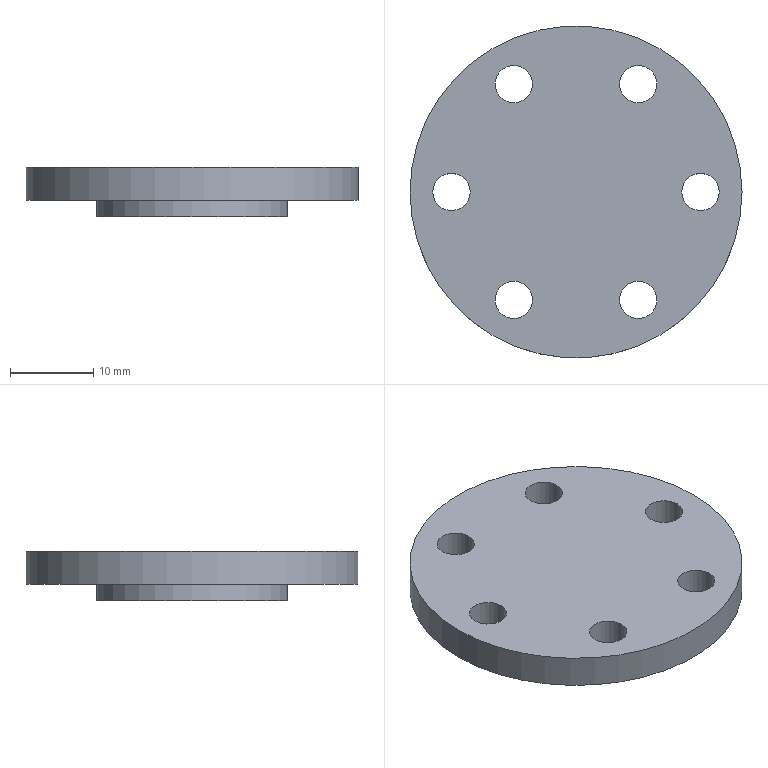Part | STEP file | zhouchenyagai2 | 1 solid | 13 faces | box 40 x 40 x 6 mm | volume 4909 mm3 | cylinder 9 | plane 4 | commonest cylinder face diameters 4.5 x6 19 x1 23 x1 40 x1
STEP:
#1=CARTESIAN_POINT('',(0.,0.,0.));
#2=DIRECTION('',(0.,0.,1.));
#3=DIRECTION('',(1.,0.,0.));
#4=AXIS2_PLACEMENT_3D('',#1,#2,#3);
#5=CARTESIAN_POINT('',(-9.75,12.99,4.));
#6=VERTEX_POINT('',#5);
#7=CARTESIAN_POINT('',(-7.5,12.99,4.));
#8=DIRECTION('',(0.,0.,-1.));
#9=DIRECTION('',(-1.,0.,0.));
#10=AXIS2_PLACEMENT_3D('',#7,#8,#9);
#11=CIRCLE('',#10,2.25);
#12=CARTESIAN_POINT('',(0.,0.,4.));
#13=DIRECTION('',(0.,0.,1.));
#14=DIRECTION('',(1.,0.,0.));
#15=AXIS2_PLACEMENT_3D('',#12,#13,#14);
#16=PLANE('',#15);
#17=CARTESIAN_POINT('',(-9.75,12.99));
#18=CARTESIAN_POINT('',(-9.75,16.887));
#19=CARTESIAN_POINT('',(-6.375,14.939));
#20=CARTESIAN_POINT('',(-3.,12.99));
#21=CARTESIAN_POINT('',(-6.375,11.042));
#22=CARTESIAN_POINT('',(-9.75,9.093));
#23=CARTESIAN_POINT('',(-9.75,12.99));
#24=(BOUNDED_CURVE()B_SPLINE_CURVE(2,(#17,#18,#19,#20,#21,#22,#23),.UNSPECIFIED.,.T.,.F.)B_SPLINE_CURVE_WITH_KNOTS((1,2,2,2,2,1),(-2.094,0.,2.094,4.189,6.283,8.378),.UNSPECIFIED.)CURVE()GEOMETRIC_REPRESENTATION_ITEM()RATIONAL_B_SPLINE_CURVE((1.,0.5,1.,0.5,1.,0.5,1.))REPRESENTATION_ITEM(''));
#25=(GEOMETRIC_REPRESENTATION_CONTEXT(2)PARAMETRIC_REPRESENTATION_CONTEXT()REPRESENTATION_CONTEXT('',''));
#26=DEFINITIONAL_REPRESENTATION('',(#24),#25);
#27=PCURVE('',#16,#26);
#28=CARTESIAN_POINT('',(-7.5,12.99,4.));
#29=DIRECTION('',(0.,0.,-1.));
#30=DIRECTION('',(-1.,0.,0.));
#31=AXIS2_PLACEMENT_3D('',#28,#29,#30);
#32=CYLINDRICAL_SURFACE('',#31,2.25);
#33=CARTESIAN_POINT('',(0.,0.));
#34=DIRECTION('',(1.,0.));
#35=VECTOR('',#34,1.);
#36=LINE('',#33,#35);
#37=(GEOMETRIC_REPRESENTATION_CONTEXT(2)PARAMETRIC_REPRESENTATION_CONTEXT()REPRESENTATION_CONTEXT('',''));
#38=DEFINITIONAL_REPRESENTATION('',(#36),#37);
#39=PCURVE('',#32,#38);
#40=SURFACE_CURVE('',#11,(#27,#39),.PCURVE_S1.);
#41=EDGE_CURVE('',#6,#6,#40,.T.);
#42=ORIENTED_EDGE('',*,*,#41,.T.);
#43=EDGE_LOOP('',(#42));
#44=FACE_BOUND('',#43,.T.);
#45=CARTESIAN_POINT('',(12.75,0.,4.));
#46=VERTEX_POINT('',#45);
#47=CARTESIAN_POINT('',(15.,0.,4.));
#48=DIRECTION('',(0.,0.,-1.));
#49=DIRECTION('',(-1.,0.,0.));
#50=AXIS2_PLACEMENT_3D('',#47,#48,#49);
#51=CIRCLE('',#50,2.25);
#52=CARTESIAN_POINT('',(12.75,0.));
#53=CARTESIAN_POINT('',(12.75,3.897));
#54=CARTESIAN_POINT('',(16.125,1.949));
#55=CARTESIAN_POINT('',(19.5,0.));
#56=CARTESIAN_POINT('',(16.125,-1.949));
#57=CARTESIAN_POINT('',(12.75,-3.897));
#58=CARTESIAN_POINT('',(12.75,0.));
#59=(BOUNDED_CURVE()B_SPLINE_CURVE(2,(#52,#53,#54,#55,#56,#57,#58),.UNSPECIFIED.,.T.,.F.)B_SPLINE_CURVE_WITH_KNOTS((1,2,2,2,2,1),(-2.094,0.,2.094,4.189,6.283,8.378),.UNSPECIFIED.)CURVE()GEOMETRIC_REPRESENTATION_ITEM()RATIONAL_B_SPLINE_CURVE((1.,0.5,1.,0.5,1.,0.5,1.))REPRESENTATION_ITEM(''));
#60=(GEOMETRIC_REPRESENTATION_CONTEXT(2)PARAMETRIC_REPRESENTATION_CONTEXT()REPRESENTATION_CONTEXT('',''));
#61=DEFINITIONAL_REPRESENTATION('',(#59),#60);
#62=PCURVE('',#16,#61);
#63=CARTESIAN_POINT('',(15.,0.,4.));
#64=DIRECTION('',(0.,0.,-1.));
#65=DIRECTION('',(-1.,0.,0.));
#66=AXIS2_PLACEMENT_3D('',#63,#64,#65);
#67=CYLINDRICAL_SURFACE('',#66,2.25);
#68=CARTESIAN_POINT('',(0.,0.));
#69=DIRECTION('',(1.,0.));
#70=VECTOR('',#69,1.);
#71=LINE('',#68,#70);
#72=(GEOMETRIC_REPRESENTATION_CONTEXT(2)PARAMETRIC_REPRESENTATION_CONTEXT()REPRESENTATION_CONTEXT('',''));
#73=DEFINITIONAL_REPRESENTATION('',(#71),#72);
#74=PCURVE('',#67,#73);
#75=SURFACE_CURVE('',#51,(#62,#74),.PCURVE_S1.);
#76=EDGE_CURVE('',#46,#46,#75,.T.);
#77=ORIENTED_EDGE('',*,*,#76,.T.);
#78=EDGE_LOOP('',(#77));
#79=FACE_BOUND('',#78,.T.);
#80=CARTESIAN_POINT('',(-9.75,-12.99,4.));
#81=VERTEX_POINT('',#80);
#82=CARTESIAN_POINT('',(-7.5,-12.99,4.));
#83=DIRECTION('',(0.,0.,-1.));
#84=DIRECTION('',(-1.,0.,0.));
#85=AXIS2_PLACEMENT_3D('',#82,#83,#84);
#86=CIRCLE('',#85,2.25);
#87=CARTESIAN_POINT('',(-9.75,-12.99));
#88=CARTESIAN_POINT('',(-9.75,-9.093));
#89=CARTESIAN_POINT('',(-6.375,-11.042));
#90=CARTESIAN_POINT('',(-3.,-12.99));
#91=CARTESIAN_POINT('',(-6.375,-14.939));
#92=CARTESIAN_POINT('',(-9.75,-16.887));
#93=CARTESIAN_POINT('',(-9.75,-12.99));
#94=(BOUNDED_CURVE()B_SPLINE_CURVE(2,(#87,#88,#89,#90,#91,#92,#93),.UNSPECIFIED.,.T.,.F.)B_SPLINE_CURVE_WITH_KNOTS((1,2,2,2,2,1),(-2.094,0.,2.094,4.189,6.283,8.378),.UNSPECIFIED.)CURVE()GEOMETRIC_REPRESENTATION_ITEM()RATIONAL_B_SPLINE_CURVE((1.,0.5,1.,0.5,1.,0.5,1.))REPRESENTATION_ITEM(''));
#95=(GEOMETRIC_REPRESENTATION_CONTEXT(2)PARAMETRIC_REPRESENTATION_CONTEXT()REPRESENTATION_CONTEXT('',''));
#96=DEFINITIONAL_REPRESENTATION('',(#94),#95);
#97=PCURVE('',#16,#96);
#98=CARTESIAN_POINT('',(-7.5,-12.99,4.));
#99=DIRECTION('',(0.,0.,-1.));
#100=DIRECTION('',(-1.,0.,0.));
#101=AXIS2_PLACEMENT_3D('',#98,#99,#100);
#102=CYLINDRICAL_SURFACE('',#101,2.25);
#103=CARTESIAN_POINT('',(0.,0.));
#104=DIRECTION('',(1.,0.));
#105=VECTOR('',#104,1.);
#106=LINE('',#103,#105);
#107=(GEOMETRIC_REPRESENTATION_CONTEXT(2)PARAMETRIC_REPRESENTATION_CONTEXT()REPRESENTATION_CONTEXT('',''));
#108=DEFINITIONAL_REPRESENTATION('',(#106),#107);
#109=PCURVE('',#102,#108);
#110=SURFACE_CURVE('',#86,(#97,#109),.PCURVE_S1.);
#111=EDGE_CURVE('',#81,#81,#110,.T.);
#112=ORIENTED_EDGE('',*,*,#111,.T.);
#113=EDGE_LOOP('',(#112));
#114=FACE_BOUND('',#113,.T.);
#115=CARTESIAN_POINT('',(-20.,0.,4.));
#116=VERTEX_POINT('',#115);
#117=CARTESIAN_POINT('',(0.,0.,4.));
#118=DIRECTION('',(0.,0.,1.));
#119=DIRECTION('',(-1.,0.,0.));
#120=AXIS2_PLACEMENT_3D('',#117,#118,#119);
#121=CIRCLE('',#120,20.);
#122=CARTESIAN_POINT('',(0.,0.));
#123=DIRECTION('',(-1.,0.));
#124=AXIS2_PLACEMENT_2D('',#122,#123);
#125=CIRCLE('',#124,20.);
#126=(GEOMETRIC_REPRESENTATION_CONTEXT(2)PARAMETRIC_REPRESENTATION_CONTEXT()REPRESENTATION_CONTEXT('',''));
#127=DEFINITIONAL_REPRESENTATION('',(#125),#126);
#128=PCURVE('',#16,#127);
#129=CARTESIAN_POINT('',(0.,0.,4.));
#130=DIRECTION('',(0.,0.,-1.));
#131=DIRECTION('',(-1.,0.,0.));
#132=AXIS2_PLACEMENT_3D('',#129,#130,#131);
#133=CYLINDRICAL_SURFACE('',#132,20.);
#134=CARTESIAN_POINT('',(6.283,0.));
#135=DIRECTION('',(-1.,0.));
#136=VECTOR('',#135,1.);
#137=LINE('',#134,#136);
#138=(GEOMETRIC_REPRESENTATION_CONTEXT(2)PARAMETRIC_REPRESENTATION_CONTEXT()REPRESENTATION_CONTEXT('',''));
#139=DEFINITIONAL_REPRESENTATION('',(#137),#138);
#140=PCURVE('',#133,#139);
#141=SURFACE_CURVE('',#121,(#128,#140),.PCURVE_S1.);
#142=EDGE_CURVE('',#116,#116,#141,.T.);
#143=ORIENTED_EDGE('',*,*,#142,.T.);
#144=EDGE_LOOP('',(#143));
#145=FACE_BOUND('',#144,.T.);
#146=CARTESIAN_POINT('',(-17.25,0.,4.));
#147=VERTEX_POINT('',#146);
#148=CARTESIAN_POINT('',(-15.,0.,4.));
#149=DIRECTION('',(0.,0.,-1.));
#150=DIRECTION('',(-1.,0.,0.));
#151=AXIS2_PLACEMENT_3D('',#148,#149,#150);
#152=CIRCLE('',#151,2.25);
#153=CARTESIAN_POINT('',(-17.25,0.));
#154=CARTESIAN_POINT('',(-17.25,3.897));
#155=CARTESIAN_POINT('',(-13.875,1.949));
#156=CARTESIAN_POINT('',(-10.5,0.));
#157=CARTESIAN_POINT('',(-13.875,-1.949));
#158=CARTESIAN_POINT('',(-17.25,-3.897));
#159=CARTESIAN_POINT('',(-17.25,0.));
#160=(BOUNDED_CURVE()B_SPLINE_CURVE(2,(#153,#154,#155,#156,#157,#158,#159),.UNSPECIFIED.,.T.,.F.)B_SPLINE_CURVE_WITH_KNOTS((1,2,2,2,2,1),(-2.094,0.,2.094,4.189,6.283,8.378),.UNSPECIFIED.)CURVE()GEOMETRIC_REPRESENTATION_ITEM()RATIONAL_B_SPLINE_CURVE((1.,0.5,1.,0.5,1.,0.5,1.))REPRESENTATION_ITEM(''));
#161=(GEOMETRIC_REPRESENTATION_CONTEXT(2)PARAMETRIC_REPRESENTATION_CONTEXT()REPRESENTATION_CONTEXT('',''));
#162=DEFINITIONAL_REPRESENTATION('',(#160),#161);
#163=PCURVE('',#16,#162);
#164=CARTESIAN_POINT('',(-15.,0.,4.));
#165=DIRECTION('',(0.,0.,-1.));
#166=DIRECTION('',(-1.,0.,0.));
#167=AXIS2_PLACEMENT_3D('',#164,#165,#166);
#168=CYLINDRICAL_SURFACE('',#167,2.25);
#169=CARTESIAN_POINT('',(0.,0.));
#170=DIRECTION('',(1.,0.));
#171=VECTOR('',#170,1.);
#172=LINE('',#169,#171);
#173=(GEOMETRIC_REPRESENTATION_CONTEXT(2)PARAMETRIC_REPRESENTATION_CONTEXT()REPRESENTATION_CONTEXT('',''));
#174=DEFINITIONAL_REPRESENTATION('',(#172),#173);
#175=PCURVE('',#168,#174);
#176=SURFACE_CURVE('',#152,(#163,#175),.PCURVE_S1.);
#177=EDGE_CURVE('',#147,#147,#176,.T.);
#178=ORIENTED_EDGE('',*,*,#177,.T.);
#179=EDGE_LOOP('',(#178));
#180=FACE_BOUND('',#179,.T.);
#181=CARTESIAN_POINT('',(5.25,-12.99,4.));
#182=VERTEX_POINT('',#181);
#183=CARTESIAN_POINT('',(7.5,-12.99,4.));
#184=DIRECTION('',(0.,0.,-1.));
#185=DIRECTION('',(-1.,0.,0.));
#186=AXIS2_PLACEMENT_3D('',#183,#184,#185);
#187=CIRCLE('',#186,2.25);
#188=CARTESIAN_POINT('',(5.25,-12.99));
#189=CARTESIAN_POINT('',(5.25,-9.093));
#190=CARTESIAN_POINT('',(8.625,-11.042));
#191=CARTESIAN_POINT('',(12.,-12.99));
#192=CARTESIAN_POINT('',(8.625,-14.939));
#193=CARTESIAN_POINT('',(5.25,-16.887));
#194=CARTESIAN_POINT('',(5.25,-12.99));
#195=(BOUNDED_CURVE()B_SPLINE_CURVE(2,(#188,#189,#190,#191,#192,#193,#194),.UNSPECIFIED.,.T.,.F.)B_SPLINE_CURVE_WITH_KNOTS((1,2,2,2,2,1),(-2.094,0.,2.094,4.189,6.283,8.378),.UNSPECIFIED.)CURVE()GEOMETRIC_REPRESENTATION_ITEM()RATIONAL_B_SPLINE_CURVE((1.,0.5,1.,0.5,1.,0.5,1.))REPRESENTATION_ITEM(''));
#196=(GEOMETRIC_REPRESENTATION_CONTEXT(2)PARAMETRIC_REPRESENTATION_CONTEXT()REPRESENTATION_CONTEXT('',''));
#197=DEFINITIONAL_REPRESENTATION('',(#195),#196);
#198=PCURVE('',#16,#197);
#199=CARTESIAN_POINT('',(7.5,-12.99,4.));
#200=DIRECTION('',(0.,0.,-1.));
#201=DIRECTION('',(-1.,0.,0.));
#202=AXIS2_PLACEMENT_3D('',#199,#200,#201);
#203=CYLINDRICAL_SURFACE('',#202,2.25);
#204=CARTESIAN_POINT('',(0.,0.));
#205=DIRECTION('',(1.,0.));
#206=VECTOR('',#205,1.);
#207=LINE('',#204,#206);
#208=(GEOMETRIC_REPRESENTATION_CONTEXT(2)PARAMETRIC_REPRESENTATION_CONTEXT()REPRESENTATION_CONTEXT('',''));
#209=DEFINITIONAL_REPRESENTATION('',(#207),#208);
#210=PCURVE('',#203,#209);
#211=SURFACE_CURVE('',#187,(#198,#210),.PCURVE_S1.);
#212=EDGE_CURVE('',#182,#182,#211,.T.);
#213=ORIENTED_EDGE('',*,*,#212,.T.);
#214=EDGE_LOOP('',(#213));
#215=FACE_BOUND('',#214,.T.);
#216=CARTESIAN_POINT('',(5.25,12.99,4.));
#217=VERTEX_POINT('',#216);
#218=CARTESIAN_POINT('',(7.5,12.99,4.));
#219=DIRECTION('',(0.,0.,-1.));
#220=DIRECTION('',(-1.,0.,0.));
#221=AXIS2_PLACEMENT_3D('',#218,#219,#220);
#222=CIRCLE('',#221,2.25);
#223=CARTESIAN_POINT('',(5.25,12.99));
#224=CARTESIAN_POINT('',(5.25,16.887));
#225=CARTESIAN_POINT('',(8.625,14.939));
#226=CARTESIAN_POINT('',(12.,12.99));
#227=CARTESIAN_POINT('',(8.625,11.042));
#228=CARTESIAN_POINT('',(5.25,9.093));
#229=CARTESIAN_POINT('',(5.25,12.99));
#230=(BOUNDED_CURVE()B_SPLINE_CURVE(2,(#223,#224,#225,#226,#227,#228,#229),.UNSPECIFIED.,.T.,.F.)B_SPLINE_CURVE_WITH_KNOTS((1,2,2,2,2,1),(-2.094,0.,2.094,4.189,6.283,8.378),.UNSPECIFIED.)CURVE()GEOMETRIC_REPRESENTATION_ITEM()RATIONAL_B_SPLINE_CURVE((1.,0.5,1.,0.5,1.,0.5,1.))REPRESENTATION_ITEM(''));
#231=(GEOMETRIC_REPRESENTATION_CONTEXT(2)PARAMETRIC_REPRESENTATION_CONTEXT()REPRESENTATION_CONTEXT('',''));
#232=DEFINITIONAL_REPRESENTATION('',(#230),#231);
#233=PCURVE('',#16,#232);
#234=CARTESIAN_POINT('',(7.5,12.99,4.));
#235=DIRECTION('',(0.,0.,-1.));
#236=DIRECTION('',(-1.,0.,0.));
#237=AXIS2_PLACEMENT_3D('',#234,#235,#236);
#238=CYLINDRICAL_SURFACE('',#237,2.25);
#239=CARTESIAN_POINT('',(0.,0.));
#240=DIRECTION('',(1.,0.));
#241=VECTOR('',#240,1.);
#242=LINE('',#239,#241);
#243=(GEOMETRIC_REPRESENTATION_CONTEXT(2)PARAMETRIC_REPRESENTATION_CONTEXT()REPRESENTATION_CONTEXT('',''));
#244=DEFINITIONAL_REPRESENTATION('',(#242),#243);
#245=PCURVE('',#238,#244);
#246=SURFACE_CURVE('',#222,(#233,#245),.PCURVE_S1.);
#247=EDGE_CURVE('',#217,#217,#246,.T.);
#248=ORIENTED_EDGE('',*,*,#247,.T.);
#249=EDGE_LOOP('',(#248));
#250=FACE_BOUND('',#249,.T.);
#251=ADVANCED_FACE('',(#44,#79,#114,#145,#180,#215,#250),#16,.T.);
#252=ORIENTED_EDGE('',*,*,#41,.T.);
#253=CARTESIAN_POINT('',(-9.75,12.99,0.));
#254=VERTEX_POINT('',#253);
#255=CARTESIAN_POINT('',(-9.75,12.99,4.));
#256=CARTESIAN_POINT('',(-9.75,12.99,0.));
#257=B_SPLINE_CURVE_WITH_KNOTS('',1,(#255,#256),.UNSPECIFIED.,.F.,.F.,(2,2),(0.,4.),.PIECEWISE_BEZIER_KNOTS.);
#258=CARTESIAN_POINT('',(6.283,0.));
#259=DIRECTION('',(0.,1.));
#260=VECTOR('',#259,1.);
#261=LINE('',#258,#260);
#262=(GEOMETRIC_REPRESENTATION_CONTEXT(2)PARAMETRIC_REPRESENTATION_CONTEXT()REPRESENTATION_CONTEXT('',''));
#263=DEFINITIONAL_REPRESENTATION('',(#261),#262);
#264=PCURVE('',#32,#263);
#265=CARTESIAN_POINT('',(0.,0.));
#266=DIRECTION('',(0.,1.));
#267=VECTOR('',#266,1.);
#268=LINE('',#265,#267);
#269=(GEOMETRIC_REPRESENTATION_CONTEXT(2)PARAMETRIC_REPRESENTATION_CONTEXT()REPRESENTATION_CONTEXT('',''));
#270=DEFINITIONAL_REPRESENTATION('',(#268),#269);
#271=PCURVE('',#32,#270);
#272=SEAM_CURVE('',#257,(#264,#271),.PCURVE_S1.);
#273=EDGE_CURVE('',#6,#254,#272,.T.);
#274=ORIENTED_EDGE('',*,*,#273,.T.);
#275=CARTESIAN_POINT('',(-7.5,12.99,0.));
#276=DIRECTION('',(0.,0.,1.));
#277=DIRECTION('',(-1.,0.,0.));
#278=AXIS2_PLACEMENT_3D('',#275,#276,#277);
#279=CIRCLE('',#278,2.25);
#280=CARTESIAN_POINT('',(6.283,4.));
#281=DIRECTION('',(-1.,0.));
#282=VECTOR('',#281,1.);
#283=LINE('',#280,#282);
#284=(GEOMETRIC_REPRESENTATION_CONTEXT(2)PARAMETRIC_REPRESENTATION_CONTEXT()REPRESENTATION_CONTEXT('',''));
#285=DEFINITIONAL_REPRESENTATION('',(#283),#284);
#286=PCURVE('',#32,#285);
#287=CARTESIAN_POINT('',(0.,0.,0.));
#288=DIRECTION('',(0.,0.,1.));
#289=DIRECTION('',(1.,0.,0.));
#290=AXIS2_PLACEMENT_3D('',#287,#288,#289);
#291=PLANE('',#290);
#292=CARTESIAN_POINT('',(-7.5,12.99));
#293=DIRECTION('',(-1.,0.));
#294=AXIS2_PLACEMENT_2D('',#292,#293);
#295=CIRCLE('',#294,2.25);
#296=(GEOMETRIC_REPRESENTATION_CONTEXT(2)PARAMETRIC_REPRESENTATION_CONTEXT()REPRESENTATION_CONTEXT('',''));
#297=DEFINITIONAL_REPRESENTATION('',(#295),#296);
#298=PCURVE('',#291,#297);
#299=SURFACE_CURVE('',#279,(#286,#298),.PCURVE_S1.);
#300=EDGE_CURVE('',#254,#254,#299,.T.);
#301=ORIENTED_EDGE('',*,*,#300,.T.);
#302=ORIENTED_EDGE('',*,*,#273,.F.);
#303=EDGE_LOOP('',(#252,#274,#301,#302));
#304=FACE_BOUND('',#303,.F.);
#305=ADVANCED_FACE('',(#304),#32,.F.);
#306=ORIENTED_EDGE('',*,*,#76,.T.);
#307=CARTESIAN_POINT('',(12.75,0.,0.));
#308=VERTEX_POINT('',#307);
#309=CARTESIAN_POINT('',(12.75,0.,4.));
#310=CARTESIAN_POINT('',(12.75,0.,0.));
#311=B_SPLINE_CURVE_WITH_KNOTS('',1,(#309,#310),.UNSPECIFIED.,.F.,.F.,(2,2),(0.,4.),.PIECEWISE_BEZIER_KNOTS.);
#312=CARTESIAN_POINT('',(6.283,0.));
#313=DIRECTION('',(0.,1.));
#314=VECTOR('',#313,1.);
#315=LINE('',#312,#314);
#316=(GEOMETRIC_REPRESENTATION_CONTEXT(2)PARAMETRIC_REPRESENTATION_CONTEXT()REPRESENTATION_CONTEXT('',''));
#317=DEFINITIONAL_REPRESENTATION('',(#315),#316);
#318=PCURVE('',#67,#317);
#319=CARTESIAN_POINT('',(0.,0.));
#320=DIRECTION('',(0.,1.));
#321=VECTOR('',#320,1.);
#322=LINE('',#319,#321);
#323=(GEOMETRIC_REPRESENTATION_CONTEXT(2)PARAMETRIC_REPRESENTATION_CONTEXT()REPRESENTATION_CONTEXT('',''));
#324=DEFINITIONAL_REPRESENTATION('',(#322),#323);
#325=PCURVE('',#67,#324);
#326=SEAM_CURVE('',#311,(#318,#325),.PCURVE_S1.);
#327=EDGE_CURVE('',#46,#308,#326,.T.);
#328=ORIENTED_EDGE('',*,*,#327,.T.);
#329=CARTESIAN_POINT('',(15.,0.,0.));
#330=DIRECTION('',(0.,0.,1.));
#331=DIRECTION('',(-1.,0.,0.));
#332=AXIS2_PLACEMENT_3D('',#329,#330,#331);
#333=CIRCLE('',#332,2.25);
#334=CARTESIAN_POINT('',(6.283,4.));
#335=DIRECTION('',(-1.,0.));
#336=VECTOR('',#335,1.);
#337=LINE('',#334,#336);
#338=(GEOMETRIC_REPRESENTATION_CONTEXT(2)PARAMETRIC_REPRESENTATION_CONTEXT()REPRESENTATION_CONTEXT('',''));
#339=DEFINITIONAL_REPRESENTATION('',(#337),#338);
#340=PCURVE('',#67,#339);
#341=CARTESIAN_POINT('',(15.,0.));
#342=DIRECTION('',(-1.,0.));
#343=AXIS2_PLACEMENT_2D('',#341,#342);
#344=CIRCLE('',#343,2.25);
#345=(GEOMETRIC_REPRESENTATION_CONTEXT(2)PARAMETRIC_REPRESENTATION_CONTEXT()REPRESENTATION_CONTEXT('',''));
#346=DEFINITIONAL_REPRESENTATION('',(#344),#345);
#347=PCURVE('',#291,#346);
#348=SURFACE_CURVE('',#333,(#340,#347),.PCURVE_S1.);
#349=EDGE_CURVE('',#308,#308,#348,.T.);
#350=ORIENTED_EDGE('',*,*,#349,.T.);
#351=ORIENTED_EDGE('',*,*,#327,.F.);
#352=EDGE_LOOP('',(#306,#328,#350,#351));
#353=FACE_BOUND('',#352,.F.);
#354=ADVANCED_FACE('',(#353),#67,.F.);
#355=ORIENTED_EDGE('',*,*,#111,.T.);
#356=CARTESIAN_POINT('',(-9.75,-12.99,0.));
#357=VERTEX_POINT('',#356);
#358=CARTESIAN_POINT('',(-9.75,-12.99,4.));
#359=CARTESIAN_POINT('',(-9.75,-12.99,0.));
#360=B_SPLINE_CURVE_WITH_KNOTS('',1,(#358,#359),.UNSPECIFIED.,.F.,.F.,(2,2),(0.,4.),.PIECEWISE_BEZIER_KNOTS.);
#361=CARTESIAN_POINT('',(6.283,0.));
#362=DIRECTION('',(0.,1.));
#363=VECTOR('',#362,1.);
#364=LINE('',#361,#363);
#365=(GEOMETRIC_REPRESENTATION_CONTEXT(2)PARAMETRIC_REPRESENTATION_CONTEXT()REPRESENTATION_CONTEXT('',''));
#366=DEFINITIONAL_REPRESENTATION('',(#364),#365);
#367=PCURVE('',#102,#366);
#368=CARTESIAN_POINT('',(0.,0.));
#369=DIRECTION('',(0.,1.));
#370=VECTOR('',#369,1.);
#371=LINE('',#368,#370);
#372=(GEOMETRIC_REPRESENTATION_CONTEXT(2)PARAMETRIC_REPRESENTATION_CONTEXT()REPRESENTATION_CONTEXT('',''));
#373=DEFINITIONAL_REPRESENTATION('',(#371),#372);
#374=PCURVE('',#102,#373);
#375=SEAM_CURVE('',#360,(#367,#374),.PCURVE_S1.);
#376=EDGE_CURVE('',#81,#357,#375,.T.);
#377=ORIENTED_EDGE('',*,*,#376,.T.);
#378=CARTESIAN_POINT('',(-7.5,-12.99,0.));
#379=DIRECTION('',(0.,0.,1.));
#380=DIRECTION('',(-1.,0.,0.));
#381=AXIS2_PLACEMENT_3D('',#378,#379,#380);
#382=CIRCLE('',#381,2.25);
#383=CARTESIAN_POINT('',(6.283,4.));
#384=DIRECTION('',(-1.,0.));
#385=VECTOR('',#384,1.);
#386=LINE('',#383,#385);
#387=(GEOMETRIC_REPRESENTATION_CONTEXT(2)PARAMETRIC_REPRESENTATION_CONTEXT()REPRESENTATION_CONTEXT('',''));
#388=DEFINITIONAL_REPRESENTATION('',(#386),#387);
#389=PCURVE('',#102,#388);
#390=CARTESIAN_POINT('',(-7.5,-12.99));
#391=DIRECTION('',(-1.,0.));
#392=AXIS2_PLACEMENT_2D('',#390,#391);
#393=CIRCLE('',#392,2.25);
#394=(GEOMETRIC_REPRESENTATION_CONTEXT(2)PARAMETRIC_REPRESENTATION_CONTEXT()REPRESENTATION_CONTEXT('',''));
#395=DEFINITIONAL_REPRESENTATION('',(#393),#394);
#396=PCURVE('',#291,#395);
#397=SURFACE_CURVE('',#382,(#389,#396),.PCURVE_S1.);
#398=EDGE_CURVE('',#357,#357,#397,.T.);
#399=ORIENTED_EDGE('',*,*,#398,.T.);
#400=ORIENTED_EDGE('',*,*,#376,.F.);
#401=EDGE_LOOP('',(#355,#377,#399,#400));
#402=FACE_BOUND('',#401,.F.);
#403=ADVANCED_FACE('',(#402),#102,.F.);
#404=CARTESIAN_POINT('',(-20.,0.,0.));
#405=VERTEX_POINT('',#404);
#406=CARTESIAN_POINT('',(0.,0.,0.));
#407=DIRECTION('',(0.,0.,1.));
#408=DIRECTION('',(-1.,0.,0.));
#409=AXIS2_PLACEMENT_3D('',#406,#407,#408);
#410=CIRCLE('',#409,20.);
#411=CARTESIAN_POINT('',(6.283,4.));
#412=DIRECTION('',(-1.,0.));
#413=VECTOR('',#412,1.);
#414=LINE('',#411,#413);
#415=(GEOMETRIC_REPRESENTATION_CONTEXT(2)PARAMETRIC_REPRESENTATION_CONTEXT()REPRESENTATION_CONTEXT('',''));
#416=DEFINITIONAL_REPRESENTATION('',(#414),#415);
#417=PCURVE('',#133,#416);
#418=CARTESIAN_POINT('',(0.,0.));
#419=DIRECTION('',(-1.,0.));
#420=AXIS2_PLACEMENT_2D('',#418,#419);
#421=CIRCLE('',#420,20.);
#422=(GEOMETRIC_REPRESENTATION_CONTEXT(2)PARAMETRIC_REPRESENTATION_CONTEXT()REPRESENTATION_CONTEXT('',''));
#423=DEFINITIONAL_REPRESENTATION('',(#421),#422);
#424=PCURVE('',#291,#423);
#425=SURFACE_CURVE('',#410,(#417,#424),.PCURVE_S1.);
#426=EDGE_CURVE('',#405,#405,#425,.T.);
#427=ORIENTED_EDGE('',*,*,#426,.T.);
#428=CARTESIAN_POINT('',(-20.,0.,4.));
#429=CARTESIAN_POINT('',(-20.,0.,0.));
#430=B_SPLINE_CURVE_WITH_KNOTS('',1,(#428,#429),.UNSPECIFIED.,.F.,.F.,(2,2),(0.,4.),.PIECEWISE_BEZIER_KNOTS.);
#431=CARTESIAN_POINT('',(0.,0.));
#432=DIRECTION('',(0.,1.));
#433=VECTOR('',#432,1.);
#434=LINE('',#431,#433);
#435=(GEOMETRIC_REPRESENTATION_CONTEXT(2)PARAMETRIC_REPRESENTATION_CONTEXT()REPRESENTATION_CONTEXT('',''));
#436=DEFINITIONAL_REPRESENTATION('',(#434),#435);
#437=PCURVE('',#133,#436);
#438=CARTESIAN_POINT('',(6.283,0.));
#439=DIRECTION('',(0.,1.));
#440=VECTOR('',#439,1.);
#441=LINE('',#438,#440);
#442=(GEOMETRIC_REPRESENTATION_CONTEXT(2)PARAMETRIC_REPRESENTATION_CONTEXT()REPRESENTATION_CONTEXT('',''));
#443=DEFINITIONAL_REPRESENTATION('',(#441),#442);
#444=PCURVE('',#133,#443);
#445=SEAM_CURVE('',#430,(#437,#444),.PCURVE_S1.);
#446=EDGE_CURVE('',#116,#405,#445,.T.);
#447=ORIENTED_EDGE('',*,*,#446,.F.);
#448=ORIENTED_EDGE('',*,*,#142,.F.);
#449=ORIENTED_EDGE('',*,*,#446,.T.);
#450=EDGE_LOOP('',(#427,#447,#448,#449));
#451=FACE_BOUND('',#450,.T.);
#452=ADVANCED_FACE('',(#451),#133,.T.);
#453=ORIENTED_EDGE('',*,*,#177,.T.);
#454=CARTESIAN_POINT('',(-17.25,0.,0.));
#455=VERTEX_POINT('',#454);
#456=CARTESIAN_POINT('',(-17.25,0.,4.));
#457=CARTESIAN_POINT('',(-17.25,0.,0.));
#458=B_SPLINE_CURVE_WITH_KNOTS('',1,(#456,#457),.UNSPECIFIED.,.F.,.F.,(2,2),(0.,4.),.PIECEWISE_BEZIER_KNOTS.);
#459=CARTESIAN_POINT('',(6.283,0.));
#460=DIRECTION('',(0.,1.));
#461=VECTOR('',#460,1.);
#462=LINE('',#459,#461);
#463=(GEOMETRIC_REPRESENTATION_CONTEXT(2)PARAMETRIC_REPRESENTATION_CONTEXT()REPRESENTATION_CONTEXT('',''));
#464=DEFINITIONAL_REPRESENTATION('',(#462),#463);
#465=PCURVE('',#168,#464);
#466=CARTESIAN_POINT('',(0.,0.));
#467=DIRECTION('',(0.,1.));
#468=VECTOR('',#467,1.);
#469=LINE('',#466,#468);
#470=(GEOMETRIC_REPRESENTATION_CONTEXT(2)PARAMETRIC_REPRESENTATION_CONTEXT()REPRESENTATION_CONTEXT('',''));
#471=DEFINITIONAL_REPRESENTATION('',(#469),#470);
#472=PCURVE('',#168,#471);
#473=SEAM_CURVE('',#458,(#465,#472),.PCURVE_S1.);
#474=EDGE_CURVE('',#147,#455,#473,.T.);
#475=ORIENTED_EDGE('',*,*,#474,.T.);
#476=CARTESIAN_POINT('',(-15.,0.,0.));
#477=DIRECTION('',(0.,0.,1.));
#478=DIRECTION('',(-1.,0.,0.));
#479=AXIS2_PLACEMENT_3D('',#476,#477,#478);
#480=CIRCLE('',#479,2.25);
#481=CARTESIAN_POINT('',(6.283,4.));
#482=DIRECTION('',(-1.,0.));
#483=VECTOR('',#482,1.);
#484=LINE('',#481,#483);
#485=(GEOMETRIC_REPRESENTATION_CONTEXT(2)PARAMETRIC_REPRESENTATION_CONTEXT()REPRESENTATION_CONTEXT('',''));
#486=DEFINITIONAL_REPRESENTATION('',(#484),#485);
#487=PCURVE('',#168,#486);
#488=CARTESIAN_POINT('',(-15.,0.));
#489=DIRECTION('',(-1.,0.));
#490=AXIS2_PLACEMENT_2D('',#488,#489);
#491=CIRCLE('',#490,2.25);
#492=(GEOMETRIC_REPRESENTATION_CONTEXT(2)PARAMETRIC_REPRESENTATION_CONTEXT()REPRESENTATION_CONTEXT('',''));
#493=DEFINITIONAL_REPRESENTATION('',(#491),#492);
#494=PCURVE('',#291,#493);
#495=SURFACE_CURVE('',#480,(#487,#494),.PCURVE_S1.);
#496=EDGE_CURVE('',#455,#455,#495,.T.);
#497=ORIENTED_EDGE('',*,*,#496,.T.);
#498=ORIENTED_EDGE('',*,*,#474,.F.);
#499=EDGE_LOOP('',(#453,#475,#497,#498));
#500=FACE_BOUND('',#499,.F.);
#501=ADVANCED_FACE('',(#500),#168,.F.);
#502=ORIENTED_EDGE('',*,*,#212,.T.);
#503=CARTESIAN_POINT('',(5.25,-12.99,0.));
#504=VERTEX_POINT('',#503);
#505=CARTESIAN_POINT('',(5.25,-12.99,4.));
#506=CARTESIAN_POINT('',(5.25,-12.99,0.));
#507=B_SPLINE_CURVE_WITH_KNOTS('',1,(#505,#506),.UNSPECIFIED.,.F.,.F.,(2,2),(0.,4.),.PIECEWISE_BEZIER_KNOTS.);
#508=CARTESIAN_POINT('',(6.283,0.));
#509=DIRECTION('',(0.,1.));
#510=VECTOR('',#509,1.);
#511=LINE('',#508,#510);
#512=(GEOMETRIC_REPRESENTATION_CONTEXT(2)PARAMETRIC_REPRESENTATION_CONTEXT()REPRESENTATION_CONTEXT('',''));
#513=DEFINITIONAL_REPRESENTATION('',(#511),#512);
#514=PCURVE('',#203,#513);
#515=CARTESIAN_POINT('',(0.,0.));
#516=DIRECTION('',(0.,1.));
#517=VECTOR('',#516,1.);
#518=LINE('',#515,#517);
#519=(GEOMETRIC_REPRESENTATION_CONTEXT(2)PARAMETRIC_REPRESENTATION_CONTEXT()REPRESENTATION_CONTEXT('',''));
#520=DEFINITIONAL_REPRESENTATION('',(#518),#519);
#521=PCURVE('',#203,#520);
#522=SEAM_CURVE('',#507,(#514,#521),.PCURVE_S1.);
#523=EDGE_CURVE('',#182,#504,#522,.T.);
#524=ORIENTED_EDGE('',*,*,#523,.T.);
#525=CARTESIAN_POINT('',(7.5,-12.99,0.));
#526=DIRECTION('',(0.,0.,1.));
#527=DIRECTION('',(-1.,0.,0.));
#528=AXIS2_PLACEMENT_3D('',#525,#526,#527);
#529=CIRCLE('',#528,2.25);
#530=CARTESIAN_POINT('',(6.283,4.));
#531=DIRECTION('',(-1.,0.));
#532=VECTOR('',#531,1.);
#533=LINE('',#530,#532);
#534=(GEOMETRIC_REPRESENTATION_CONTEXT(2)PARAMETRIC_REPRESENTATION_CONTEXT()REPRESENTATION_CONTEXT('',''));
#535=DEFINITIONAL_REPRESENTATION('',(#533),#534);
#536=PCURVE('',#203,#535);
#537=CARTESIAN_POINT('',(7.5,-12.99));
#538=DIRECTION('',(-1.,0.));
#539=AXIS2_PLACEMENT_2D('',#537,#538);
#540=CIRCLE('',#539,2.25);
#541=(GEOMETRIC_REPRESENTATION_CONTEXT(2)PARAMETRIC_REPRESENTATION_CONTEXT()REPRESENTATION_CONTEXT('',''));
#542=DEFINITIONAL_REPRESENTATION('',(#540),#541);
#543=PCURVE('',#291,#542);
#544=SURFACE_CURVE('',#529,(#536,#543),.PCURVE_S1.);
#545=EDGE_CURVE('',#504,#504,#544,.T.);
#546=ORIENTED_EDGE('',*,*,#545,.T.);
#547=ORIENTED_EDGE('',*,*,#523,.F.);
#548=EDGE_LOOP('',(#502,#524,#546,#547));
#549=FACE_BOUND('',#548,.F.);
#550=ADVANCED_FACE('',(#549),#203,.F.);
#551=ORIENTED_EDGE('',*,*,#247,.T.);
#552=CARTESIAN_POINT('',(5.25,12.99,0.));
#553=VERTEX_POINT('',#552);
#554=CARTESIAN_POINT('',(5.25,12.99,4.));
#555=CARTESIAN_POINT('',(5.25,12.99,0.));
#556=B_SPLINE_CURVE_WITH_KNOTS('',1,(#554,#555),.UNSPECIFIED.,.F.,.F.,(2,2),(0.,4.),.PIECEWISE_BEZIER_KNOTS.);
#557=CARTESIAN_POINT('',(6.283,0.));
#558=DIRECTION('',(0.,1.));
#559=VECTOR('',#558,1.);
#560=LINE('',#557,#559);
#561=(GEOMETRIC_REPRESENTATION_CONTEXT(2)PARAMETRIC_REPRESENTATION_CONTEXT()REPRESENTATION_CONTEXT('',''));
#562=DEFINITIONAL_REPRESENTATION('',(#560),#561);
#563=PCURVE('',#238,#562);
#564=CARTESIAN_POINT('',(0.,0.));
#565=DIRECTION('',(0.,1.));
#566=VECTOR('',#565,1.);
#567=LINE('',#564,#566);
#568=(GEOMETRIC_REPRESENTATION_CONTEXT(2)PARAMETRIC_REPRESENTATION_CONTEXT()REPRESENTATION_CONTEXT('',''));
#569=DEFINITIONAL_REPRESENTATION('',(#567),#568);
#570=PCURVE('',#238,#569);
#571=SEAM_CURVE('',#556,(#563,#570),.PCURVE_S1.);
#572=EDGE_CURVE('',#217,#553,#571,.T.);
#573=ORIENTED_EDGE('',*,*,#572,.T.);
#574=CARTESIAN_POINT('',(7.5,12.99,0.));
#575=DIRECTION('',(0.,0.,1.));
#576=DIRECTION('',(-1.,0.,0.));
#577=AXIS2_PLACEMENT_3D('',#574,#575,#576);
#578=CIRCLE('',#577,2.25);
#579=CARTESIAN_POINT('',(6.283,4.));
#580=DIRECTION('',(-1.,0.));
#581=VECTOR('',#580,1.);
#582=LINE('',#579,#581);
#583=(GEOMETRIC_REPRESENTATION_CONTEXT(2)PARAMETRIC_REPRESENTATION_CONTEXT()REPRESENTATION_CONTEXT('',''));
#584=DEFINITIONAL_REPRESENTATION('',(#582),#583);
#585=PCURVE('',#238,#584);
#586=CARTESIAN_POINT('',(7.5,12.99));
#587=DIRECTION('',(-1.,0.));
#588=AXIS2_PLACEMENT_2D('',#586,#587);
#589=CIRCLE('',#588,2.25);
#590=(GEOMETRIC_REPRESENTATION_CONTEXT(2)PARAMETRIC_REPRESENTATION_CONTEXT()REPRESENTATION_CONTEXT('',''));
#591=DEFINITIONAL_REPRESENTATION('',(#589),#590);
#592=PCURVE('',#291,#591);
#593=SURFACE_CURVE('',#578,(#585,#592),.PCURVE_S1.);
#594=EDGE_CURVE('',#553,#553,#593,.T.);
#595=ORIENTED_EDGE('',*,*,#594,.T.);
#596=ORIENTED_EDGE('',*,*,#572,.F.);
#597=EDGE_LOOP('',(#551,#573,#595,#596));
#598=FACE_BOUND('',#597,.F.);
#599=ADVANCED_FACE('',(#598),#238,.F.);
#600=ORIENTED_EDGE('',*,*,#300,.T.);
#601=EDGE_LOOP('',(#600));
#602=FACE_BOUND('',#601,.T.);
#603=ORIENTED_EDGE('',*,*,#594,.T.);
#604=EDGE_LOOP('',(#603));
#605=FACE_BOUND('',#604,.T.);
#606=ORIENTED_EDGE('',*,*,#349,.T.);
#607=EDGE_LOOP('',(#606));
#608=FACE_BOUND('',#607,.T.);
#609=ORIENTED_EDGE('',*,*,#545,.T.);
#610=EDGE_LOOP('',(#609));
#611=FACE_BOUND('',#610,.T.);
#612=ORIENTED_EDGE('',*,*,#398,.T.);
#613=EDGE_LOOP('',(#612));
#614=FACE_BOUND('',#613,.T.);
#615=ORIENTED_EDGE('',*,*,#496,.T.);
#616=EDGE_LOOP('',(#615));
#617=FACE_BOUND('',#616,.T.);
#618=ORIENTED_EDGE('',*,*,#426,.F.);
#619=EDGE_LOOP('',(#618));
#620=FACE_BOUND('',#619,.T.);
#621=CARTESIAN_POINT('',(11.5,0.,0.));
#622=VERTEX_POINT('',#621);
#623=CARTESIAN_POINT('',(0.,0.,0.));
#624=DIRECTION('',(0.,0.,-1.));
#625=DIRECTION('',(1.,0.,0.));
#626=AXIS2_PLACEMENT_3D('',#623,#624,#625);
#627=CIRCLE('',#626,11.5);
#628=CARTESIAN_POINT('',(11.5,0.));
#629=CARTESIAN_POINT('',(11.5,-19.919));
#630=CARTESIAN_POINT('',(-5.75,-9.959));
#631=CARTESIAN_POINT('',(-23.,0.));
#632=CARTESIAN_POINT('',(-5.75,9.959));
#633=CARTESIAN_POINT('',(11.5,19.919));
#634=CARTESIAN_POINT('',(11.5,0.));
#635=(BOUNDED_CURVE()B_SPLINE_CURVE(2,(#628,#629,#630,#631,#632,#633,#634),.UNSPECIFIED.,.T.,.F.)B_SPLINE_CURVE_WITH_KNOTS((1,2,2,2,2,1),(-2.094,0.,2.094,4.189,6.283,8.378),.UNSPECIFIED.)CURVE()GEOMETRIC_REPRESENTATION_ITEM()RATIONAL_B_SPLINE_CURVE((1.,0.5,1.,0.5,1.,0.5,1.))REPRESENTATION_ITEM(''));
#636=(GEOMETRIC_REPRESENTATION_CONTEXT(2)PARAMETRIC_REPRESENTATION_CONTEXT()REPRESENTATION_CONTEXT('',''));
#637=DEFINITIONAL_REPRESENTATION('',(#635),#636);
#638=PCURVE('',#291,#637);
#639=CARTESIAN_POINT('',(0.,0.,-2.));
#640=DIRECTION('',(0.,0.,1.));
#641=DIRECTION('',(1.,0.,0.));
#642=AXIS2_PLACEMENT_3D('',#639,#640,#641);
#643=CYLINDRICAL_SURFACE('',#642,11.5);
#644=CARTESIAN_POINT('',(6.283,2.));
#645=DIRECTION('',(-1.,0.));
#646=VECTOR('',#645,1.);
#647=LINE('',#644,#646);
#648=(GEOMETRIC_REPRESENTATION_CONTEXT(2)PARAMETRIC_REPRESENTATION_CONTEXT()REPRESENTATION_CONTEXT('',''));
#649=DEFINITIONAL_REPRESENTATION('',(#647),#648);
#650=PCURVE('',#643,#649);
#651=SURFACE_CURVE('',#627,(#638,#650),.PCURVE_S1.);
#652=EDGE_CURVE('',#622,#622,#651,.T.);
#653=ORIENTED_EDGE('',*,*,#652,.F.);
#654=EDGE_LOOP('',(#653));
#655=FACE_BOUND('',#654,.T.);
#656=ADVANCED_FACE('',(#602,#605,#608,#611,#614,#617,#620,#655),#291,.F.);
#657=CARTESIAN_POINT('',(11.5,0.,-2.));
#658=VERTEX_POINT('',#657);
#659=CARTESIAN_POINT('',(0.,0.,-2.));
#660=DIRECTION('',(0.,0.,1.));
#661=DIRECTION('',(1.,0.,0.));
#662=AXIS2_PLACEMENT_3D('',#659,#660,#661);
#663=CIRCLE('',#662,11.5);
#664=CARTESIAN_POINT('',(0.,0.));
#665=DIRECTION('',(1.,0.));
#666=VECTOR('',#665,1.);
#667=LINE('',#664,#666);
#668=(GEOMETRIC_REPRESENTATION_CONTEXT(2)PARAMETRIC_REPRESENTATION_CONTEXT()REPRESENTATION_CONTEXT('',''));
#669=DEFINITIONAL_REPRESENTATION('',(#667),#668);
#670=PCURVE('',#643,#669);
#671=CARTESIAN_POINT('',(0.,0.,-2.));
#672=DIRECTION('',(0.,0.,-1.));
#673=DIRECTION('',(-1.,0.,0.));
#674=AXIS2_PLACEMENT_3D('',#671,#672,#673);
#675=PLANE('',#674);
#676=CARTESIAN_POINT('',(-11.5,0.));
#677=CARTESIAN_POINT('',(-11.5,19.919));
#678=CARTESIAN_POINT('',(5.75,9.959));
#679=CARTESIAN_POINT('',(23.,0.));
#680=CARTESIAN_POINT('',(5.75,-9.959));
#681=CARTESIAN_POINT('',(-11.5,-19.919));
#682=CARTESIAN_POINT('',(-11.5,0.));
#683=(BOUNDED_CURVE()B_SPLINE_CURVE(2,(#676,#677,#678,#679,#680,#681,#682),.UNSPECIFIED.,.T.,.F.)B_SPLINE_CURVE_WITH_KNOTS((1,2,2,2,2,1),(-2.094,0.,2.094,4.189,6.283,8.378),.UNSPECIFIED.)CURVE()GEOMETRIC_REPRESENTATION_ITEM()RATIONAL_B_SPLINE_CURVE((1.,0.5,1.,0.5,1.,0.5,1.))REPRESENTATION_ITEM(''));
#684=(GEOMETRIC_REPRESENTATION_CONTEXT(2)PARAMETRIC_REPRESENTATION_CONTEXT()REPRESENTATION_CONTEXT('',''));
#685=DEFINITIONAL_REPRESENTATION('',(#683),#684);
#686=PCURVE('',#675,#685);
#687=SURFACE_CURVE('',#663,(#670,#686),.PCURVE_S1.);
#688=EDGE_CURVE('',#658,#658,#687,.T.);
#689=ORIENTED_EDGE('',*,*,#688,.T.);
#690=CARTESIAN_POINT('',(11.5,0.,-2.));
#691=CARTESIAN_POINT('',(11.5,0.,0.));
#692=B_SPLINE_CURVE_WITH_KNOTS('',1,(#690,#691),.UNSPECIFIED.,.F.,.F.,(2,2),(0.,2.),.PIECEWISE_BEZIER_KNOTS.);
#693=CARTESIAN_POINT('',(6.283,0.));
#694=DIRECTION('',(0.,1.));
#695=VECTOR('',#694,1.);
#696=LINE('',#693,#695);
#697=(GEOMETRIC_REPRESENTATION_CONTEXT(2)PARAMETRIC_REPRESENTATION_CONTEXT()REPRESENTATION_CONTEXT('',''));
#698=DEFINITIONAL_REPRESENTATION('',(#696),#697);
#699=PCURVE('',#643,#698);
#700=CARTESIAN_POINT('',(0.,0.));
#701=DIRECTION('',(0.,1.));
#702=VECTOR('',#701,1.);
#703=LINE('',#700,#702);
#704=(GEOMETRIC_REPRESENTATION_CONTEXT(2)PARAMETRIC_REPRESENTATION_CONTEXT()REPRESENTATION_CONTEXT('',''));
#705=DEFINITIONAL_REPRESENTATION('',(#703),#704);
#706=PCURVE('',#643,#705);
#707=SEAM_CURVE('',#692,(#699,#706),.PCURVE_S1.);
#708=EDGE_CURVE('',#658,#622,#707,.T.);
#709=ORIENTED_EDGE('',*,*,#708,.T.);
#710=ORIENTED_EDGE('',*,*,#652,.T.);
#711=ORIENTED_EDGE('',*,*,#708,.F.);
#712=EDGE_LOOP('',(#689,#709,#710,#711));
#713=FACE_BOUND('',#712,.T.);
#714=ADVANCED_FACE('',(#713),#643,.T.);
#715=CARTESIAN_POINT('',(9.5,0.,-2.));
#716=VERTEX_POINT('',#715);
#717=CARTESIAN_POINT('',(0.,0.,-2.));
#718=DIRECTION('',(0.,0.,1.));
#719=DIRECTION('',(1.,0.,0.));
#720=AXIS2_PLACEMENT_3D('',#717,#718,#719);
#721=CIRCLE('',#720,9.5);
#722=CARTESIAN_POINT('',(-9.5,0.));
#723=CARTESIAN_POINT('',(-9.5,16.454));
#724=CARTESIAN_POINT('',(4.75,8.227));
#725=CARTESIAN_POINT('',(19.,0.));
#726=CARTESIAN_POINT('',(4.75,-8.227));
#727=CARTESIAN_POINT('',(-9.5,-16.454));
#728=CARTESIAN_POINT('',(-9.5,0.));
#729=(BOUNDED_CURVE()B_SPLINE_CURVE(2,(#722,#723,#724,#725,#726,#727,#728),.UNSPECIFIED.,.T.,.F.)B_SPLINE_CURVE_WITH_KNOTS((1,2,2,2,2,1),(-2.094,0.,2.094,4.189,6.283,8.378),.UNSPECIFIED.)CURVE()GEOMETRIC_REPRESENTATION_ITEM()RATIONAL_B_SPLINE_CURVE((1.,0.5,1.,0.5,1.,0.5,1.))REPRESENTATION_ITEM(''));
#730=(GEOMETRIC_REPRESENTATION_CONTEXT(2)PARAMETRIC_REPRESENTATION_CONTEXT()REPRESENTATION_CONTEXT('',''));
#731=DEFINITIONAL_REPRESENTATION('',(#729),#730);
#732=PCURVE('',#675,#731);
#733=CARTESIAN_POINT('',(0.,0.,-2.));
#734=DIRECTION('',(0.,0.,1.));
#735=DIRECTION('',(1.,0.,0.));
#736=AXIS2_PLACEMENT_3D('',#733,#734,#735);
#737=CYLINDRICAL_SURFACE('',#736,9.5);
#738=CARTESIAN_POINT('',(0.,0.));
#739=DIRECTION('',(1.,0.));
#740=VECTOR('',#739,1.);
#741=LINE('',#738,#740);
#742=(GEOMETRIC_REPRESENTATION_CONTEXT(2)PARAMETRIC_REPRESENTATION_CONTEXT()REPRESENTATION_CONTEXT('',''));
#743=DEFINITIONAL_REPRESENTATION('',(#741),#742);
#744=PCURVE('',#737,#743);
#745=SURFACE_CURVE('',#721,(#732,#744),.PCURVE_S1.);
#746=EDGE_CURVE('',#716,#716,#745,.T.);
#747=ORIENTED_EDGE('',*,*,#746,.T.);
#748=EDGE_LOOP('',(#747));
#749=FACE_BOUND('',#748,.T.);
#750=ORIENTED_EDGE('',*,*,#688,.F.);
#751=EDGE_LOOP('',(#750));
#752=FACE_BOUND('',#751,.T.);
#753=ADVANCED_FACE('',(#749,#752),#675,.T.);
#754=ORIENTED_EDGE('',*,*,#746,.T.);
#755=CARTESIAN_POINT('',(9.5,0.,0.));
#756=VERTEX_POINT('',#755);
#757=CARTESIAN_POINT('',(9.5,0.,-2.));
#758=CARTESIAN_POINT('',(9.5,0.,0.));
#759=B_SPLINE_CURVE_WITH_KNOTS('',1,(#757,#758),.UNSPECIFIED.,.F.,.F.,(2,2),(0.,2.),.PIECEWISE_BEZIER_KNOTS.);
#760=CARTESIAN_POINT('',(6.283,0.));
#761=DIRECTION('',(0.,1.));
#762=VECTOR('',#761,1.);
#763=LINE('',#760,#762);
#764=(GEOMETRIC_REPRESENTATION_CONTEXT(2)PARAMETRIC_REPRESENTATION_CONTEXT()REPRESENTATION_CONTEXT('',''));
#765=DEFINITIONAL_REPRESENTATION('',(#763),#764);
#766=PCURVE('',#737,#765);
#767=CARTESIAN_POINT('',(0.,0.));
#768=DIRECTION('',(0.,1.));
#769=VECTOR('',#768,1.);
#770=LINE('',#767,#769);
#771=(GEOMETRIC_REPRESENTATION_CONTEXT(2)PARAMETRIC_REPRESENTATION_CONTEXT()REPRESENTATION_CONTEXT('',''));
#772=DEFINITIONAL_REPRESENTATION('',(#770),#771);
#773=PCURVE('',#737,#772);
#774=SEAM_CURVE('',#759,(#766,#773),.PCURVE_S1.);
#775=EDGE_CURVE('',#716,#756,#774,.T.);
#776=ORIENTED_EDGE('',*,*,#775,.T.);
#777=CARTESIAN_POINT('',(0.,0.,0.));
#778=DIRECTION('',(0.,0.,-1.));
#779=DIRECTION('',(1.,0.,0.));
#780=AXIS2_PLACEMENT_3D('',#777,#778,#779);
#781=CIRCLE('',#780,9.5);
#782=CARTESIAN_POINT('',(6.283,2.));
#783=DIRECTION('',(-1.,0.));
#784=VECTOR('',#783,1.);
#785=LINE('',#782,#784);
#786=(GEOMETRIC_REPRESENTATION_CONTEXT(2)PARAMETRIC_REPRESENTATION_CONTEXT()REPRESENTATION_CONTEXT('',''));
#787=DEFINITIONAL_REPRESENTATION('',(#785),#786);
#788=PCURVE('',#737,#787);
#789=CARTESIAN_POINT('',(0.,0.,0.));
#790=DIRECTION('',(0.,0.,1.));
#791=DIRECTION('',(1.,0.,0.));
#792=AXIS2_PLACEMENT_3D('',#789,#790,#791);
#793=PLANE('',#792);
#794=CARTESIAN_POINT('',(9.5,0.));
#795=CARTESIAN_POINT('',(9.5,-16.454));
#796=CARTESIAN_POINT('',(-4.75,-8.227));
#797=CARTESIAN_POINT('',(-19.,0.));
#798=CARTESIAN_POINT('',(-4.75,8.227));
#799=CARTESIAN_POINT('',(9.5,16.454));
#800=CARTESIAN_POINT('',(9.5,0.));
#801=(BOUNDED_CURVE()B_SPLINE_CURVE(2,(#794,#795,#796,#797,#798,#799,#800),.UNSPECIFIED.,.T.,.F.)B_SPLINE_CURVE_WITH_KNOTS((1,2,2,2,2,1),(-2.094,0.,2.094,4.189,6.283,8.378),.UNSPECIFIED.)CURVE()GEOMETRIC_REPRESENTATION_ITEM()RATIONAL_B_SPLINE_CURVE((1.,0.5,1.,0.5,1.,0.5,1.))REPRESENTATION_ITEM(''));
#802=(GEOMETRIC_REPRESENTATION_CONTEXT(2)PARAMETRIC_REPRESENTATION_CONTEXT()REPRESENTATION_CONTEXT('',''));
#803=DEFINITIONAL_REPRESENTATION('',(#801),#802);
#804=PCURVE('',#793,#803);
#805=SURFACE_CURVE('',#781,(#788,#804),.PCURVE_S1.);
#806=EDGE_CURVE('',#756,#756,#805,.T.);
#807=ORIENTED_EDGE('',*,*,#806,.T.);
#808=ORIENTED_EDGE('',*,*,#775,.F.);
#809=EDGE_LOOP('',(#754,#776,#807,#808));
#810=FACE_BOUND('',#809,.F.);
#811=ADVANCED_FACE('',(#810),#737,.F.);
#812=ORIENTED_EDGE('',*,*,#806,.T.);
#813=EDGE_LOOP('',(#812));
#814=FACE_BOUND('',#813,.T.);
#815=ADVANCED_FACE('',(#814),#793,.F.);
#816=CLOSED_SHELL('',(#251,#305,#354,#403,#452,#501,#550,#599,#656,#714,#753,#811,#815));
#817=MANIFOLD_SOLID_BREP('',#816);
#818=(LENGTH_UNIT()NAMED_UNIT(*)SI_UNIT(.MILLI.,.METRE.));
#819=UNCERTAINTY_MEASURE_WITH_UNIT(LENGTH_MEASURE(0.00001),#818,'','');
#820=(NAMED_UNIT(*)PLANE_ANGLE_UNIT()SI_UNIT($,.RADIAN.));
#821=(NAMED_UNIT(*)SI_UNIT($,.STERADIAN.)SOLID_ANGLE_UNIT());
#822=(GEOMETRIC_REPRESENTATION_CONTEXT(3)GLOBAL_UNCERTAINTY_ASSIGNED_CONTEXT((#819))GLOBAL_UNIT_ASSIGNED_CONTEXT((#818,#820,#821))REPRESENTATION_CONTEXT('',''));
#823=ADVANCED_BREP_SHAPE_REPRESENTATION('',(#4,#817),#822);